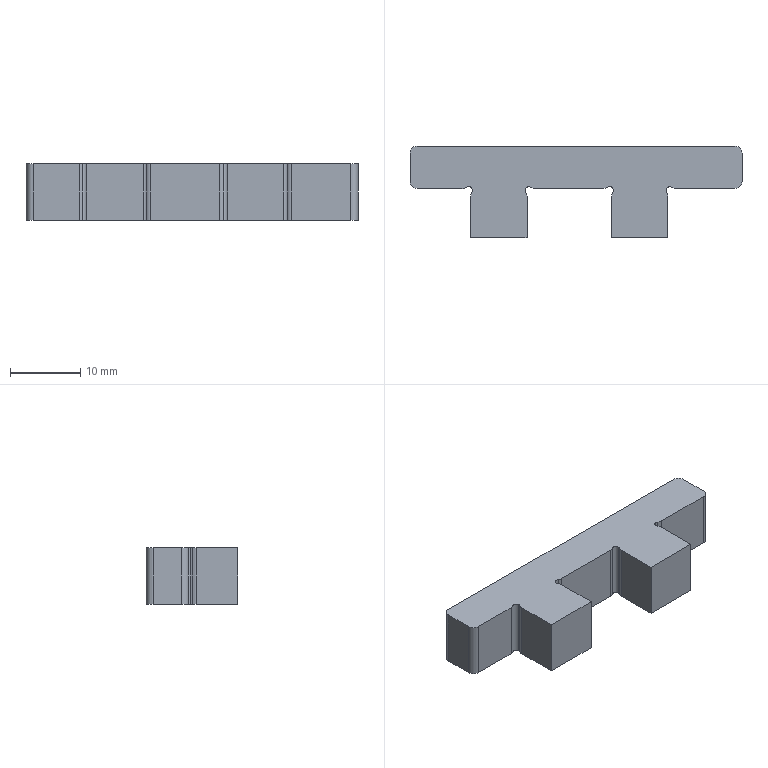Part | SolidWorks | features Fillet 1, FlatPattern 1, ICE 1, SMBaseFlange 1, SheetMetal 1 | 1 solid | 32 faces | box 47.1 x 13 x 8 mm | volume 3140 mm3 | cylinder 18 | plane 14 | commonest cylinder face diameters 2 x12 1 x6
STEP:
#1=CARTESIAN_POINT('',(-10.518,-33.899,0.));
#2=VERTEX_POINT('',#1);
#3=CARTESIAN_POINT('',(-11.295,-33.482,0.));
#4=VERTEX_POINT('',#3);
#5=CARTESIAN_POINT('',(-11.018,-33.899,0.));
#6=DIRECTION('',(0.,0.,1.));
#7=DIRECTION('',(1.,0.,0.));
#8=AXIS2_PLACEMENT_3D('',#5,#6,#7);
#9=CIRCLE('',#8,0.5);
#10=EDGE_CURVE('',#2,#4,#9,.T.);
#11=ORIENTED_EDGE('',*,*,#10,.F.);
#12=CARTESIAN_POINT('',(-10.518,-33.899,8.));
#13=VERTEX_POINT('',#12);
#14=CARTESIAN_POINT('',(-10.518,-33.899,0.));
#15=DIRECTION('',(0.,0.,1.));
#16=VECTOR('',#15,1000.);
#17=LINE('',#14,#16);
#18=EDGE_CURVE('',#2,#13,#17,.T.);
#19=ORIENTED_EDGE('',*,*,#18,.T.);
#20=CARTESIAN_POINT('',(-11.295,-33.482,8.));
#21=VERTEX_POINT('',#20);
#22=CARTESIAN_POINT('',(-11.018,-33.899,8.));
#23=DIRECTION('',(0.,0.,1.));
#24=DIRECTION('',(1.,0.,0.));
#25=AXIS2_PLACEMENT_3D('',#22,#23,#24);
#26=CIRCLE('',#25,0.5);
#27=EDGE_CURVE('',#13,#21,#26,.T.);
#28=ORIENTED_EDGE('',*,*,#27,.T.);
#29=CARTESIAN_POINT('',(-11.295,-33.482,0.));
#30=DIRECTION('',(0.,0.,-1.));
#31=VECTOR('',#30,1000.);
#32=LINE('',#29,#31);
#33=EDGE_CURVE('',#21,#4,#32,.T.);
#34=ORIENTED_EDGE('',*,*,#33,.T.);
#35=EDGE_LOOP('',(#11,#19,#28,#34));
#36=FACE_OUTER_BOUND('',#35,.T.);
#37=CARTESIAN_POINT('',(-11.018,-33.899,0.));
#38=DIRECTION('',(0.,0.,1.));
#39=DIRECTION('',(1.,0.,0.));
#40=AXIS2_PLACEMENT_3D('',#37,#38,#39);
#41=CYLINDRICAL_SURFACE('',#40,0.5);
#42=ADVANCED_FACE('',(#36),#41,.F.);
#43=CARTESIAN_POINT('',(9.482,-33.899,0.));
#44=VERTEX_POINT('',#43);
#45=CARTESIAN_POINT('',(8.705,-33.482,0.));
#46=VERTEX_POINT('',#45);
#47=CARTESIAN_POINT('',(8.982,-33.899,0.));
#48=DIRECTION('',(0.,0.,1.));
#49=DIRECTION('',(1.,0.,0.));
#50=AXIS2_PLACEMENT_3D('',#47,#48,#49);
#51=CIRCLE('',#50,0.5);
#52=EDGE_CURVE('',#44,#46,#51,.T.);
#53=ORIENTED_EDGE('',*,*,#52,.F.);
#54=CARTESIAN_POINT('',(9.482,-33.899,8.));
#55=VERTEX_POINT('',#54);
#56=CARTESIAN_POINT('',(9.482,-33.899,0.));
#57=DIRECTION('',(0.,0.,1.));
#58=VECTOR('',#57,1000.);
#59=LINE('',#56,#58);
#60=EDGE_CURVE('',#44,#55,#59,.T.);
#61=ORIENTED_EDGE('',*,*,#60,.T.);
#62=CARTESIAN_POINT('',(8.705,-33.482,8.));
#63=VERTEX_POINT('',#62);
#64=CARTESIAN_POINT('',(8.982,-33.899,8.));
#65=DIRECTION('',(0.,0.,1.));
#66=DIRECTION('',(1.,0.,0.));
#67=AXIS2_PLACEMENT_3D('',#64,#65,#66);
#68=CIRCLE('',#67,0.5);
#69=EDGE_CURVE('',#55,#63,#68,.T.);
#70=ORIENTED_EDGE('',*,*,#69,.T.);
#71=CARTESIAN_POINT('',(8.705,-33.482,0.));
#72=DIRECTION('',(0.,0.,-1.));
#73=VECTOR('',#72,1000.);
#74=LINE('',#71,#73);
#75=EDGE_CURVE('',#63,#46,#74,.T.);
#76=ORIENTED_EDGE('',*,*,#75,.T.);
#77=EDGE_LOOP('',(#53,#61,#70,#76));
#78=FACE_OUTER_BOUND('',#77,.T.);
#79=CARTESIAN_POINT('',(8.982,-33.899,0.));
#80=DIRECTION('',(0.,0.,1.));
#81=DIRECTION('',(1.,0.,0.));
#82=AXIS2_PLACEMENT_3D('',#79,#80,#81);
#83=CYLINDRICAL_SURFACE('',#82,0.5);
#84=ADVANCED_FACE('',(#78),#83,.F.);
#85=CARTESIAN_POINT('',(-18.368,-33.649,8.));
#86=VERTEX_POINT('',#85);
#87=CARTESIAN_POINT('',(-11.847,-33.649,8.));
#88=VERTEX_POINT('',#87);
#89=CARTESIAN_POINT('',(-10.768,-33.649,8.));
#90=DIRECTION('',(1.,0.,0.));
#91=VECTOR('',#90,1000.);
#92=LINE('',#89,#91);
#93=EDGE_CURVE('',#86,#88,#92,.T.);
#94=ORIENTED_EDGE('',*,*,#93,.F.);
#95=CARTESIAN_POINT('',(-18.368,-33.649,0.));
#96=VERTEX_POINT('',#95);
#97=CARTESIAN_POINT('',(-18.368,-33.649,8.));
#98=DIRECTION('',(0.,0.,-1.));
#99=VECTOR('',#98,1000.);
#100=LINE('',#97,#99);
#101=EDGE_CURVE('',#86,#96,#100,.T.);
#102=ORIENTED_EDGE('',*,*,#101,.T.);
#103=CARTESIAN_POINT('',(-11.847,-33.649,0.));
#104=VERTEX_POINT('',#103);
#105=CARTESIAN_POINT('',(-10.768,-33.649,0.));
#106=DIRECTION('',(1.,0.,0.));
#107=VECTOR('',#106,1000.);
#108=LINE('',#105,#107);
#109=EDGE_CURVE('',#96,#104,#108,.T.);
#110=ORIENTED_EDGE('',*,*,#109,.T.);
#111=CARTESIAN_POINT('',(-11.847,-33.649,8.));
#112=DIRECTION('',(0.,0.,1.));
#113=VECTOR('',#112,1000.);
#114=LINE('',#111,#113);
#115=EDGE_CURVE('',#104,#88,#114,.T.);
#116=ORIENTED_EDGE('',*,*,#115,.T.);
#117=EDGE_LOOP('',(#94,#102,#110,#116));
#118=FACE_OUTER_BOUND('',#117,.T.);
#119=CARTESIAN_POINT('',(-10.768,-33.649,8.));
#120=DIRECTION('',(0.,1.,0.));
#121=DIRECTION('',(0.,0.,1.));
#122=AXIS2_PLACEMENT_3D('',#119,#120,#121);
#123=PLANE('',#122);
#124=ADVANCED_FACE('',(#118),#123,.F.);
#125=CARTESIAN_POINT('',(-10.768,-34.728,8.));
#126=VERTEX_POINT('',#125);
#127=CARTESIAN_POINT('',(-10.768,-40.649,8.));
#128=VERTEX_POINT('',#127);
#129=CARTESIAN_POINT('',(-10.768,-40.649,8.));
#130=DIRECTION('',(0.,-1.,0.));
#131=VECTOR('',#130,1000.);
#132=LINE('',#129,#131);
#133=EDGE_CURVE('',#126,#128,#132,.T.);
#134=ORIENTED_EDGE('',*,*,#133,.F.);
#135=CARTESIAN_POINT('',(-10.768,-34.728,0.));
#136=VERTEX_POINT('',#135);
#137=CARTESIAN_POINT('',(-10.768,-34.728,0.));
#138=DIRECTION('',(0.,0.,-1.));
#139=VECTOR('',#138,1000.);
#140=LINE('',#137,#139);
#141=EDGE_CURVE('',#126,#136,#140,.T.);
#142=ORIENTED_EDGE('',*,*,#141,.T.);
#143=CARTESIAN_POINT('',(-10.768,-40.649,0.));
#144=VERTEX_POINT('',#143);
#145=CARTESIAN_POINT('',(-10.768,-40.649,0.));
#146=DIRECTION('',(0.,-1.,0.));
#147=VECTOR('',#146,1000.);
#148=LINE('',#145,#147);
#149=EDGE_CURVE('',#136,#144,#148,.T.);
#150=ORIENTED_EDGE('',*,*,#149,.T.);
#151=CARTESIAN_POINT('',(-10.768,-40.649,8.));
#152=DIRECTION('',(0.,0.,-1.));
#153=VECTOR('',#152,1000.);
#154=LINE('',#151,#153);
#155=EDGE_CURVE('',#128,#144,#154,.T.);
#156=ORIENTED_EDGE('',*,*,#155,.F.);
#157=EDGE_LOOP('',(#134,#142,#150,#156));
#158=FACE_OUTER_BOUND('',#157,.T.);
#159=CARTESIAN_POINT('',(-10.768,-40.649,8.));
#160=DIRECTION('',(1.,0.,0.));
#161=DIRECTION('',(0.,0.,-1.));
#162=AXIS2_PLACEMENT_3D('',#159,#160,#161);
#163=PLANE('',#162);
#164=ADVANCED_FACE('',(#158),#163,.F.);
#165=CARTESIAN_POINT('',(-2.768,-40.649,0.));
#166=VERTEX_POINT('',#165);
#167=CARTESIAN_POINT('',(-2.768,-34.728,0.));
#168=VERTEX_POINT('',#167);
#169=CARTESIAN_POINT('',(-2.768,-33.649,0.));
#170=DIRECTION('',(0.,1.,0.));
#171=VECTOR('',#170,1000.);
#172=LINE('',#169,#171);
#173=EDGE_CURVE('',#166,#168,#172,.T.);
#174=ORIENTED_EDGE('',*,*,#173,.T.);
#175=CARTESIAN_POINT('',(-2.768,-34.728,8.));
#176=VERTEX_POINT('',#175);
#177=CARTESIAN_POINT('',(-2.768,-34.728,8.));
#178=DIRECTION('',(0.,0.,1.));
#179=VECTOR('',#178,1000.);
#180=LINE('',#177,#179);
#181=EDGE_CURVE('',#168,#176,#180,.T.);
#182=ORIENTED_EDGE('',*,*,#181,.T.);
#183=CARTESIAN_POINT('',(-2.768,-40.649,8.));
#184=VERTEX_POINT('',#183);
#185=CARTESIAN_POINT('',(-2.768,-33.649,8.));
#186=DIRECTION('',(0.,1.,0.));
#187=VECTOR('',#186,1000.);
#188=LINE('',#185,#187);
#189=EDGE_CURVE('',#184,#176,#188,.T.);
#190=ORIENTED_EDGE('',*,*,#189,.F.);
#191=CARTESIAN_POINT('',(-2.768,-40.649,8.));
#192=DIRECTION('',(0.,0.,-1.));
#193=VECTOR('',#192,1000.);
#194=LINE('',#191,#193);
#195=EDGE_CURVE('',#184,#166,#194,.T.);
#196=ORIENTED_EDGE('',*,*,#195,.T.);
#197=EDGE_LOOP('',(#174,#182,#190,#196));
#198=FACE_OUTER_BOUND('',#197,.T.);
#199=CARTESIAN_POINT('',(-2.768,-33.649,8.));
#200=DIRECTION('',(-1.,0.,0.));
#201=DIRECTION('',(0.,0.,1.));
#202=AXIS2_PLACEMENT_3D('',#199,#200,#201);
#203=PLANE('',#202);
#204=ADVANCED_FACE('',(#198),#203,.F.);
#205=CARTESIAN_POINT('',(-1.689,-33.649,0.));
#206=VERTEX_POINT('',#205);
#207=CARTESIAN_POINT('',(8.153,-33.649,0.));
#208=VERTEX_POINT('',#207);
#209=CARTESIAN_POINT('',(9.232,-33.649,0.));
#210=DIRECTION('',(1.,0.,0.));
#211=VECTOR('',#210,1000.);
#212=LINE('',#209,#211);
#213=EDGE_CURVE('',#206,#208,#212,.T.);
#214=ORIENTED_EDGE('',*,*,#213,.T.);
#215=CARTESIAN_POINT('',(8.153,-33.649,8.));
#216=VERTEX_POINT('',#215);
#217=CARTESIAN_POINT('',(8.153,-33.649,8.));
#218=DIRECTION('',(0.,0.,1.));
#219=VECTOR('',#218,1000.);
#220=LINE('',#217,#219);
#221=EDGE_CURVE('',#208,#216,#220,.T.);
#222=ORIENTED_EDGE('',*,*,#221,.T.);
#223=CARTESIAN_POINT('',(-1.689,-33.649,8.));
#224=VERTEX_POINT('',#223);
#225=CARTESIAN_POINT('',(9.232,-33.649,8.));
#226=DIRECTION('',(1.,0.,0.));
#227=VECTOR('',#226,1000.);
#228=LINE('',#225,#227);
#229=EDGE_CURVE('',#224,#216,#228,.T.);
#230=ORIENTED_EDGE('',*,*,#229,.F.);
#231=CARTESIAN_POINT('',(-1.689,-33.649,0.));
#232=DIRECTION('',(0.,0.,-1.));
#233=VECTOR('',#232,1000.);
#234=LINE('',#231,#233);
#235=EDGE_CURVE('',#224,#206,#234,.T.);
#236=ORIENTED_EDGE('',*,*,#235,.T.);
#237=EDGE_LOOP('',(#214,#222,#230,#236));
#238=FACE_OUTER_BOUND('',#237,.T.);
#239=CARTESIAN_POINT('',(9.232,-33.649,8.));
#240=DIRECTION('',(0.,1.,0.));
#241=DIRECTION('',(0.,0.,1.));
#242=AXIS2_PLACEMENT_3D('',#239,#240,#241);
#243=PLANE('',#242);
#244=ADVANCED_FACE('',(#238),#243,.F.);
#245=CARTESIAN_POINT('',(9.232,-34.728,8.));
#246=VERTEX_POINT('',#245);
#247=CARTESIAN_POINT('',(9.232,-40.649,8.));
#248=VERTEX_POINT('',#247);
#249=CARTESIAN_POINT('',(9.232,-40.649,8.));
#250=DIRECTION('',(0.,-1.,0.));
#251=VECTOR('',#250,1000.);
#252=LINE('',#249,#251);
#253=EDGE_CURVE('',#246,#248,#252,.T.);
#254=ORIENTED_EDGE('',*,*,#253,.F.);
#255=CARTESIAN_POINT('',(9.232,-34.728,0.));
#256=VERTEX_POINT('',#255);
#257=CARTESIAN_POINT('',(9.232,-34.728,0.));
#258=DIRECTION('',(0.,0.,-1.));
#259=VECTOR('',#258,1000.);
#260=LINE('',#257,#259);
#261=EDGE_CURVE('',#246,#256,#260,.T.);
#262=ORIENTED_EDGE('',*,*,#261,.T.);
#263=CARTESIAN_POINT('',(9.232,-40.649,0.));
#264=VERTEX_POINT('',#263);
#265=CARTESIAN_POINT('',(9.232,-40.649,0.));
#266=DIRECTION('',(0.,-1.,0.));
#267=VECTOR('',#266,1000.);
#268=LINE('',#265,#267);
#269=EDGE_CURVE('',#256,#264,#268,.T.);
#270=ORIENTED_EDGE('',*,*,#269,.T.);
#271=CARTESIAN_POINT('',(9.232,-40.649,8.));
#272=DIRECTION('',(0.,0.,-1.));
#273=VECTOR('',#272,1000.);
#274=LINE('',#271,#273);
#275=EDGE_CURVE('',#248,#264,#274,.T.);
#276=ORIENTED_EDGE('',*,*,#275,.F.);
#277=EDGE_LOOP('',(#254,#262,#270,#276));
#278=FACE_OUTER_BOUND('',#277,.T.);
#279=CARTESIAN_POINT('',(9.232,-40.649,8.));
#280=DIRECTION('',(1.,0.,0.));
#281=DIRECTION('',(0.,0.,-1.));
#282=AXIS2_PLACEMENT_3D('',#279,#280,#281);
#283=PLANE('',#282);
#284=ADVANCED_FACE('',(#278),#283,.F.);
#285=CARTESIAN_POINT('',(17.232,-40.649,0.));
#286=VERTEX_POINT('',#285);
#287=CARTESIAN_POINT('',(17.232,-34.728,0.));
#288=VERTEX_POINT('',#287);
#289=CARTESIAN_POINT('',(17.232,-33.649,0.));
#290=DIRECTION('',(0.,1.,0.));
#291=VECTOR('',#290,1000.);
#292=LINE('',#289,#291);
#293=EDGE_CURVE('',#286,#288,#292,.T.);
#294=ORIENTED_EDGE('',*,*,#293,.T.);
#295=CARTESIAN_POINT('',(17.232,-34.728,8.));
#296=VERTEX_POINT('',#295);
#297=CARTESIAN_POINT('',(17.232,-34.728,8.));
#298=DIRECTION('',(0.,0.,1.));
#299=VECTOR('',#298,1000.);
#300=LINE('',#297,#299);
#301=EDGE_CURVE('',#288,#296,#300,.T.);
#302=ORIENTED_EDGE('',*,*,#301,.T.);
#303=CARTESIAN_POINT('',(17.232,-40.649,8.));
#304=VERTEX_POINT('',#303);
#305=CARTESIAN_POINT('',(17.232,-33.649,8.));
#306=DIRECTION('',(0.,1.,0.));
#307=VECTOR('',#306,1000.);
#308=LINE('',#305,#307);
#309=EDGE_CURVE('',#304,#296,#308,.T.);
#310=ORIENTED_EDGE('',*,*,#309,.F.);
#311=CARTESIAN_POINT('',(17.232,-40.649,8.));
#312=DIRECTION('',(0.,0.,-1.));
#313=VECTOR('',#312,1000.);
#314=LINE('',#311,#313);
#315=EDGE_CURVE('',#304,#286,#314,.T.);
#316=ORIENTED_EDGE('',*,*,#315,.T.);
#317=EDGE_LOOP('',(#294,#302,#310,#316));
#318=FACE_OUTER_BOUND('',#317,.T.);
#319=CARTESIAN_POINT('',(17.232,-33.649,8.));
#320=DIRECTION('',(-1.,0.,0.));
#321=DIRECTION('',(0.,0.,1.));
#322=AXIS2_PLACEMENT_3D('',#319,#320,#321);
#323=PLANE('',#322);
#324=ADVANCED_FACE('',(#318),#323,.F.);
#325=CARTESIAN_POINT('',(18.311,-33.649,0.));
#326=VERTEX_POINT('',#325);
#327=CARTESIAN_POINT('',(26.732,-33.649,0.));
#328=VERTEX_POINT('',#327);
#329=CARTESIAN_POINT('',(27.732,-33.649,0.));
#330=DIRECTION('',(1.,0.,0.));
#331=VECTOR('',#330,1000.);
#332=LINE('',#329,#331);
#333=EDGE_CURVE('',#326,#328,#332,.T.);
#334=ORIENTED_EDGE('',*,*,#333,.T.);
#335=CARTESIAN_POINT('',(26.732,-33.649,8.));
#336=VERTEX_POINT('',#335);
#337=CARTESIAN_POINT('',(26.732,-33.649,8.));
#338=DIRECTION('',(0.,0.,1.));
#339=VECTOR('',#338,1000.);
#340=LINE('',#337,#339);
#341=EDGE_CURVE('',#328,#336,#340,.T.);
#342=ORIENTED_EDGE('',*,*,#341,.T.);
#343=CARTESIAN_POINT('',(18.311,-33.649,8.));
#344=VERTEX_POINT('',#343);
#345=CARTESIAN_POINT('',(27.732,-33.649,8.));
#346=DIRECTION('',(1.,0.,0.));
#347=VECTOR('',#346,1000.);
#348=LINE('',#345,#347);
#349=EDGE_CURVE('',#344,#336,#348,.T.);
#350=ORIENTED_EDGE('',*,*,#349,.F.);
#351=CARTESIAN_POINT('',(18.311,-33.649,0.));
#352=DIRECTION('',(0.,0.,-1.));
#353=VECTOR('',#352,1000.);
#354=LINE('',#351,#353);
#355=EDGE_CURVE('',#344,#326,#354,.T.);
#356=ORIENTED_EDGE('',*,*,#355,.T.);
#357=EDGE_LOOP('',(#334,#342,#350,#356));
#358=FACE_OUTER_BOUND('',#357,.T.);
#359=CARTESIAN_POINT('',(27.732,-33.649,8.));
#360=DIRECTION('',(0.,1.,0.));
#361=DIRECTION('',(0.,0.,1.));
#362=AXIS2_PLACEMENT_3D('',#359,#360,#361);
#363=PLANE('',#362);
#364=ADVANCED_FACE('',(#358),#363,.F.);
#365=ORIENTED_EDGE('',*,*,#349,.T.);
#366=CARTESIAN_POINT('',(27.732,-32.649,8.));
#367=VERTEX_POINT('',#366);
#368=CARTESIAN_POINT('',(26.732,-32.649,8.));
#369=DIRECTION('',(0.,0.,1.));
#370=DIRECTION('',(1.,0.,0.));
#371=AXIS2_PLACEMENT_3D('',#368,#369,#370);
#372=CIRCLE('',#371,1.);
#373=EDGE_CURVE('',#336,#367,#372,.T.);
#374=ORIENTED_EDGE('',*,*,#373,.T.);
#375=CARTESIAN_POINT('',(27.732,-28.649,8.));
#376=VERTEX_POINT('',#375);
#377=CARTESIAN_POINT('',(27.732,-27.649,8.));
#378=DIRECTION('',(0.,1.,0.));
#379=VECTOR('',#378,1000.);
#380=LINE('',#377,#379);
#381=EDGE_CURVE('',#367,#376,#380,.T.);
#382=ORIENTED_EDGE('',*,*,#381,.T.);
#383=CARTESIAN_POINT('',(26.732,-27.649,8.));
#384=VERTEX_POINT('',#383);
#385=CARTESIAN_POINT('',(26.732,-28.649,8.));
#386=DIRECTION('',(0.,0.,1.));
#387=DIRECTION('',(1.,0.,0.));
#388=AXIS2_PLACEMENT_3D('',#385,#386,#387);
#389=CIRCLE('',#388,1.);
#390=EDGE_CURVE('',#376,#384,#389,.T.);
#391=ORIENTED_EDGE('',*,*,#390,.T.);
#392=CARTESIAN_POINT('',(-18.368,-27.649,8.));
#393=VERTEX_POINT('',#392);
#394=CARTESIAN_POINT('',(-19.368,-27.649,8.));
#395=DIRECTION('',(-1.,0.,0.));
#396=VECTOR('',#395,1000.);
#397=LINE('',#394,#396);
#398=EDGE_CURVE('',#384,#393,#397,.T.);
#399=ORIENTED_EDGE('',*,*,#398,.T.);
#400=CARTESIAN_POINT('',(-19.368,-28.649,8.));
#401=VERTEX_POINT('',#400);
#402=CARTESIAN_POINT('',(-18.368,-28.649,8.));
#403=DIRECTION('',(0.,0.,1.));
#404=DIRECTION('',(1.,0.,0.));
#405=AXIS2_PLACEMENT_3D('',#402,#403,#404);
#406=CIRCLE('',#405,1.);
#407=EDGE_CURVE('',#393,#401,#406,.T.);
#408=ORIENTED_EDGE('',*,*,#407,.T.);
#409=CARTESIAN_POINT('',(-19.368,-32.649,8.));
#410=VERTEX_POINT('',#409);
#411=CARTESIAN_POINT('',(-19.368,-33.649,8.));
#412=DIRECTION('',(0.000001026,-1.,0.));
#413=VECTOR('',#412,1000.);
#414=LINE('',#411,#413);
#415=EDGE_CURVE('',#401,#410,#414,.T.);
#416=ORIENTED_EDGE('',*,*,#415,.T.);
#417=CARTESIAN_POINT('',(-18.368,-32.649,8.));
#418=DIRECTION('',(0.,0.,1.));
#419=DIRECTION('',(1.,0.,0.));
#420=AXIS2_PLACEMENT_3D('',#417,#418,#419);
#421=CIRCLE('',#420,1.);
#422=EDGE_CURVE('',#410,#86,#421,.T.);
#423=ORIENTED_EDGE('',*,*,#422,.T.);
#424=ORIENTED_EDGE('',*,*,#93,.T.);
#425=CARTESIAN_POINT('',(-11.847,-32.649,8.));
#426=DIRECTION('',(0.,0.,1.));
#427=DIRECTION('',(1.,0.,0.));
#428=AXIS2_PLACEMENT_3D('',#425,#426,#427);
#429=CIRCLE('',#428,1.);
#430=EDGE_CURVE('',#88,#21,#429,.T.);
#431=ORIENTED_EDGE('',*,*,#430,.T.);
#432=ORIENTED_EDGE('',*,*,#27,.F.);
#433=CARTESIAN_POINT('',(-10.602,-34.175,8.));
#434=VERTEX_POINT('',#433);
#435=CARTESIAN_POINT('',(-11.018,-33.899,8.));
#436=DIRECTION('',(0.,0.,1.));
#437=DIRECTION('',(1.,0.,0.));
#438=AXIS2_PLACEMENT_3D('',#435,#436,#437);
#439=CIRCLE('',#438,0.5);
#440=EDGE_CURVE('',#434,#13,#439,.T.);
#441=ORIENTED_EDGE('',*,*,#440,.F.);
#442=CARTESIAN_POINT('',(-9.768,-34.728,8.));
#443=DIRECTION('',(0.,0.,1.));
#444=DIRECTION('',(1.,0.,0.));
#445=AXIS2_PLACEMENT_3D('',#442,#443,#444);
#446=CIRCLE('',#445,1.);
#447=EDGE_CURVE('',#434,#126,#446,.T.);
#448=ORIENTED_EDGE('',*,*,#447,.T.);
#449=ORIENTED_EDGE('',*,*,#133,.T.);
#450=CARTESIAN_POINT('',(-2.768,-40.649,8.));
#451=DIRECTION('',(1.,0.,0.));
#452=VECTOR('',#451,1000.);
#453=LINE('',#450,#452);
#454=EDGE_CURVE('',#128,#184,#453,.T.);
#455=ORIENTED_EDGE('',*,*,#454,.T.);
#456=ORIENTED_EDGE('',*,*,#189,.T.);
#457=CARTESIAN_POINT('',(-2.935,-34.175,8.));
#458=VERTEX_POINT('',#457);
#459=CARTESIAN_POINT('',(-3.768,-34.728,8.));
#460=DIRECTION('',(0.,0.,1.));
#461=DIRECTION('',(1.,0.,0.));
#462=AXIS2_PLACEMENT_3D('',#459,#460,#461);
#463=CIRCLE('',#462,1.);
#464=EDGE_CURVE('',#176,#458,#463,.T.);
#465=ORIENTED_EDGE('',*,*,#464,.T.);
#466=CARTESIAN_POINT('',(-2.242,-33.482,8.));
#467=VERTEX_POINT('',#466);
#468=CARTESIAN_POINT('',(-2.518,-33.899,8.));
#469=DIRECTION('',(0.,0.,1.));
#470=DIRECTION('',(1.,0.,0.));
#471=AXIS2_PLACEMENT_3D('',#468,#469,#470);
#472=CIRCLE('',#471,0.5);
#473=EDGE_CURVE('',#467,#458,#472,.T.);
#474=ORIENTED_EDGE('',*,*,#473,.F.);
#475=CARTESIAN_POINT('',(-1.689,-32.649,8.));
#476=DIRECTION('',(0.,0.,1.));
#477=DIRECTION('',(1.,0.,0.));
#478=AXIS2_PLACEMENT_3D('',#475,#476,#477);
#479=CIRCLE('',#478,1.);
#480=EDGE_CURVE('',#467,#224,#479,.T.);
#481=ORIENTED_EDGE('',*,*,#480,.T.);
#482=ORIENTED_EDGE('',*,*,#229,.T.);
#483=CARTESIAN_POINT('',(8.153,-32.649,8.));
#484=DIRECTION('',(0.,0.,1.));
#485=DIRECTION('',(1.,0.,0.));
#486=AXIS2_PLACEMENT_3D('',#483,#484,#485);
#487=CIRCLE('',#486,1.);
#488=EDGE_CURVE('',#216,#63,#487,.T.);
#489=ORIENTED_EDGE('',*,*,#488,.T.);
#490=ORIENTED_EDGE('',*,*,#69,.F.);
#491=CARTESIAN_POINT('',(9.398,-34.175,8.));
#492=VERTEX_POINT('',#491);
#493=CARTESIAN_POINT('',(8.982,-33.899,8.));
#494=DIRECTION('',(0.,0.,1.));
#495=DIRECTION('',(1.,0.,0.));
#496=AXIS2_PLACEMENT_3D('',#493,#494,#495);
#497=CIRCLE('',#496,0.5);
#498=EDGE_CURVE('',#492,#55,#497,.T.);
#499=ORIENTED_EDGE('',*,*,#498,.F.);
#500=CARTESIAN_POINT('',(10.232,-34.728,8.));
#501=DIRECTION('',(0.,0.,1.));
#502=DIRECTION('',(1.,0.,0.));
#503=AXIS2_PLACEMENT_3D('',#500,#501,#502);
#504=CIRCLE('',#503,1.);
#505=EDGE_CURVE('',#492,#246,#504,.T.);
#506=ORIENTED_EDGE('',*,*,#505,.T.);
#507=ORIENTED_EDGE('',*,*,#253,.T.);
#508=CARTESIAN_POINT('',(17.232,-40.649,8.));
#509=DIRECTION('',(1.,0.,0.));
#510=VECTOR('',#509,1000.);
#511=LINE('',#508,#510);
#512=EDGE_CURVE('',#248,#304,#511,.T.);
#513=ORIENTED_EDGE('',*,*,#512,.T.);
#514=ORIENTED_EDGE('',*,*,#309,.T.);
#515=CARTESIAN_POINT('',(17.065,-34.175,8.));
#516=VERTEX_POINT('',#515);
#517=CARTESIAN_POINT('',(16.232,-34.728,8.));
#518=DIRECTION('',(0.,0.,1.));
#519=DIRECTION('',(1.,0.,0.));
#520=AXIS2_PLACEMENT_3D('',#517,#518,#519);
#521=CIRCLE('',#520,1.);
#522=EDGE_CURVE('',#296,#516,#521,.T.);
#523=ORIENTED_EDGE('',*,*,#522,.T.);
#524=CARTESIAN_POINT('',(17.758,-33.482,8.));
#525=VERTEX_POINT('',#524);
#526=CARTESIAN_POINT('',(17.482,-33.899,8.));
#527=DIRECTION('',(0.,0.,1.));
#528=DIRECTION('',(1.,0.,0.));
#529=AXIS2_PLACEMENT_3D('',#526,#527,#528);
#530=CIRCLE('',#529,0.5);
#531=EDGE_CURVE('',#525,#516,#530,.T.);
#532=ORIENTED_EDGE('',*,*,#531,.F.);
#533=CARTESIAN_POINT('',(18.311,-32.649,8.));
#534=DIRECTION('',(0.,0.,1.));
#535=DIRECTION('',(1.,0.,0.));
#536=AXIS2_PLACEMENT_3D('',#533,#534,#535);
#537=CIRCLE('',#536,1.);
#538=EDGE_CURVE('',#525,#344,#537,.T.);
#539=ORIENTED_EDGE('',*,*,#538,.T.);
#540=EDGE_LOOP('',(#365,#374,#382,#391,#399,#408,#416,#423,#424,#431,#432,#441,#448,#449,#455,#456,#465,#474,#481,#482,#489,#490,#499,#506,#507,#513,#514,#523,#532,#539));
#541=FACE_OUTER_BOUND('',#540,.T.);
#542=CARTESIAN_POINT('',(0.,0.,8.));
#543=DIRECTION('',(0.,0.,1.));
#544=DIRECTION('',(1.,0.,0.));
#545=AXIS2_PLACEMENT_3D('',#542,#543,#544);
#546=PLANE('',#545);
#547=ADVANCED_FACE('',(#541),#546,.T.);
#548=CARTESIAN_POINT('',(27.732,-32.649,0.));
#549=VERTEX_POINT('',#548);
#550=CARTESIAN_POINT('',(27.732,-28.649,0.));
#551=VERTEX_POINT('',#550);
#552=CARTESIAN_POINT('',(27.732,-27.649,0.));
#553=DIRECTION('',(0.,1.,0.));
#554=VECTOR('',#553,1000.);
#555=LINE('',#552,#554);
#556=EDGE_CURVE('',#549,#551,#555,.T.);
#557=ORIENTED_EDGE('',*,*,#556,.F.);
#558=CARTESIAN_POINT('',(26.732,-32.649,0.));
#559=DIRECTION('',(0.,0.,-1.));
#560=DIRECTION('',(1.,0.,0.));
#561=AXIS2_PLACEMENT_3D('',#558,#559,#560);
#562=CIRCLE('',#561,1.);
#563=EDGE_CURVE('',#549,#328,#562,.T.);
#564=ORIENTED_EDGE('',*,*,#563,.T.);
#565=ORIENTED_EDGE('',*,*,#333,.F.);
#566=CARTESIAN_POINT('',(17.758,-33.482,0.));
#567=VERTEX_POINT('',#566);
#568=CARTESIAN_POINT('',(18.311,-32.649,0.));
#569=DIRECTION('',(0.,0.,-1.));
#570=DIRECTION('',(1.,0.,0.));
#571=AXIS2_PLACEMENT_3D('',#568,#569,#570);
#572=CIRCLE('',#571,1.);
#573=EDGE_CURVE('',#326,#567,#572,.T.);
#574=ORIENTED_EDGE('',*,*,#573,.T.);
#575=CARTESIAN_POINT('',(17.065,-34.175,0.));
#576=VERTEX_POINT('',#575);
#577=CARTESIAN_POINT('',(17.482,-33.899,0.));
#578=DIRECTION('',(0.,0.,1.));
#579=DIRECTION('',(1.,0.,0.));
#580=AXIS2_PLACEMENT_3D('',#577,#578,#579);
#581=CIRCLE('',#580,0.5);
#582=EDGE_CURVE('',#567,#576,#581,.T.);
#583=ORIENTED_EDGE('',*,*,#582,.T.);
#584=CARTESIAN_POINT('',(16.232,-34.728,0.));
#585=DIRECTION('',(0.,0.,-1.));
#586=DIRECTION('',(1.,0.,0.));
#587=AXIS2_PLACEMENT_3D('',#584,#585,#586);
#588=CIRCLE('',#587,1.);
#589=EDGE_CURVE('',#576,#288,#588,.T.);
#590=ORIENTED_EDGE('',*,*,#589,.T.);
#591=ORIENTED_EDGE('',*,*,#293,.F.);
#592=CARTESIAN_POINT('',(17.232,-40.649,0.));
#593=DIRECTION('',(1.,0.,0.));
#594=VECTOR('',#593,1000.);
#595=LINE('',#592,#594);
#596=EDGE_CURVE('',#264,#286,#595,.T.);
#597=ORIENTED_EDGE('',*,*,#596,.F.);
#598=ORIENTED_EDGE('',*,*,#269,.F.);
#599=CARTESIAN_POINT('',(9.398,-34.175,0.));
#600=VERTEX_POINT('',#599);
#601=CARTESIAN_POINT('',(10.232,-34.728,0.));
#602=DIRECTION('',(0.,0.,-1.));
#603=DIRECTION('',(1.,0.,0.));
#604=AXIS2_PLACEMENT_3D('',#601,#602,#603);
#605=CIRCLE('',#604,1.);
#606=EDGE_CURVE('',#256,#600,#605,.T.);
#607=ORIENTED_EDGE('',*,*,#606,.T.);
#608=CARTESIAN_POINT('',(8.982,-33.899,0.));
#609=DIRECTION('',(0.,0.,1.));
#610=DIRECTION('',(1.,0.,0.));
#611=AXIS2_PLACEMENT_3D('',#608,#609,#610);
#612=CIRCLE('',#611,0.5);
#613=EDGE_CURVE('',#600,#44,#612,.T.);
#614=ORIENTED_EDGE('',*,*,#613,.T.);
#615=ORIENTED_EDGE('',*,*,#52,.T.);
#616=CARTESIAN_POINT('',(8.153,-32.649,0.));
#617=DIRECTION('',(0.,0.,-1.));
#618=DIRECTION('',(1.,0.,0.));
#619=AXIS2_PLACEMENT_3D('',#616,#617,#618);
#620=CIRCLE('',#619,1.);
#621=EDGE_CURVE('',#46,#208,#620,.T.);
#622=ORIENTED_EDGE('',*,*,#621,.T.);
#623=ORIENTED_EDGE('',*,*,#213,.F.);
#624=CARTESIAN_POINT('',(-2.242,-33.482,0.));
#625=VERTEX_POINT('',#624);
#626=CARTESIAN_POINT('',(-1.689,-32.649,0.));
#627=DIRECTION('',(0.,0.,-1.));
#628=DIRECTION('',(1.,0.,0.));
#629=AXIS2_PLACEMENT_3D('',#626,#627,#628);
#630=CIRCLE('',#629,1.);
#631=EDGE_CURVE('',#206,#625,#630,.T.);
#632=ORIENTED_EDGE('',*,*,#631,.T.);
#633=CARTESIAN_POINT('',(-2.935,-34.175,0.));
#634=VERTEX_POINT('',#633);
#635=CARTESIAN_POINT('',(-2.518,-33.899,0.));
#636=DIRECTION('',(0.,0.,1.));
#637=DIRECTION('',(1.,0.,0.));
#638=AXIS2_PLACEMENT_3D('',#635,#636,#637);
#639=CIRCLE('',#638,0.5);
#640=EDGE_CURVE('',#625,#634,#639,.T.);
#641=ORIENTED_EDGE('',*,*,#640,.T.);
#642=CARTESIAN_POINT('',(-3.768,-34.728,0.));
#643=DIRECTION('',(0.,0.,-1.));
#644=DIRECTION('',(1.,0.,0.));
#645=AXIS2_PLACEMENT_3D('',#642,#643,#644);
#646=CIRCLE('',#645,1.);
#647=EDGE_CURVE('',#634,#168,#646,.T.);
#648=ORIENTED_EDGE('',*,*,#647,.T.);
#649=ORIENTED_EDGE('',*,*,#173,.F.);
#650=CARTESIAN_POINT('',(-2.768,-40.649,0.));
#651=DIRECTION('',(1.,0.,0.));
#652=VECTOR('',#651,1000.);
#653=LINE('',#650,#652);
#654=EDGE_CURVE('',#144,#166,#653,.T.);
#655=ORIENTED_EDGE('',*,*,#654,.F.);
#656=ORIENTED_EDGE('',*,*,#149,.F.);
#657=CARTESIAN_POINT('',(-10.602,-34.175,0.));
#658=VERTEX_POINT('',#657);
#659=CARTESIAN_POINT('',(-9.768,-34.728,0.));
#660=DIRECTION('',(0.,0.,-1.));
#661=DIRECTION('',(1.,0.,0.));
#662=AXIS2_PLACEMENT_3D('',#659,#660,#661);
#663=CIRCLE('',#662,1.);
#664=EDGE_CURVE('',#136,#658,#663,.T.);
#665=ORIENTED_EDGE('',*,*,#664,.T.);
#666=CARTESIAN_POINT('',(-11.018,-33.899,0.));
#667=DIRECTION('',(0.,0.,1.));
#668=DIRECTION('',(1.,0.,0.));
#669=AXIS2_PLACEMENT_3D('',#666,#667,#668);
#670=CIRCLE('',#669,0.5);
#671=EDGE_CURVE('',#658,#2,#670,.T.);
#672=ORIENTED_EDGE('',*,*,#671,.T.);
#673=ORIENTED_EDGE('',*,*,#10,.T.);
#674=CARTESIAN_POINT('',(-11.847,-32.649,0.));
#675=DIRECTION('',(0.,0.,-1.));
#676=DIRECTION('',(1.,0.,0.));
#677=AXIS2_PLACEMENT_3D('',#674,#675,#676);
#678=CIRCLE('',#677,1.);
#679=EDGE_CURVE('',#4,#104,#678,.T.);
#680=ORIENTED_EDGE('',*,*,#679,.T.);
#681=ORIENTED_EDGE('',*,*,#109,.F.);
#682=CARTESIAN_POINT('',(-19.368,-32.649,0.));
#683=VERTEX_POINT('',#682);
#684=CARTESIAN_POINT('',(-18.368,-32.649,0.));
#685=DIRECTION('',(0.,0.,-1.));
#686=DIRECTION('',(1.,0.,0.));
#687=AXIS2_PLACEMENT_3D('',#684,#685,#686);
#688=CIRCLE('',#687,1.);
#689=EDGE_CURVE('',#96,#683,#688,.T.);
#690=ORIENTED_EDGE('',*,*,#689,.T.);
#691=CARTESIAN_POINT('',(-19.368,-28.649,0.));
#692=VERTEX_POINT('',#691);
#693=CARTESIAN_POINT('',(-19.368,-33.649,0.));
#694=DIRECTION('',(0.000001026,-1.,0.));
#695=VECTOR('',#694,1000.);
#696=LINE('',#693,#695);
#697=EDGE_CURVE('',#692,#683,#696,.T.);
#698=ORIENTED_EDGE('',*,*,#697,.F.);
#699=CARTESIAN_POINT('',(-18.368,-27.649,0.));
#700=VERTEX_POINT('',#699);
#701=CARTESIAN_POINT('',(-18.368,-28.649,0.));
#702=DIRECTION('',(0.,0.,-1.));
#703=DIRECTION('',(1.,0.,0.));
#704=AXIS2_PLACEMENT_3D('',#701,#702,#703);
#705=CIRCLE('',#704,1.);
#706=EDGE_CURVE('',#692,#700,#705,.T.);
#707=ORIENTED_EDGE('',*,*,#706,.T.);
#708=CARTESIAN_POINT('',(26.732,-27.649,0.));
#709=VERTEX_POINT('',#708);
#710=CARTESIAN_POINT('',(-19.368,-27.649,0.));
#711=DIRECTION('',(-1.,0.,0.));
#712=VECTOR('',#711,1000.);
#713=LINE('',#710,#712);
#714=EDGE_CURVE('',#709,#700,#713,.T.);
#715=ORIENTED_EDGE('',*,*,#714,.F.);
#716=CARTESIAN_POINT('',(26.732,-28.649,0.));
#717=DIRECTION('',(0.,0.,-1.));
#718=DIRECTION('',(1.,0.,0.));
#719=AXIS2_PLACEMENT_3D('',#716,#717,#718);
#720=CIRCLE('',#719,1.);
#721=EDGE_CURVE('',#709,#551,#720,.T.);
#722=ORIENTED_EDGE('',*,*,#721,.T.);
#723=EDGE_LOOP('',(#557,#564,#565,#574,#583,#590,#591,#597,#598,#607,#614,#615,#622,#623,#632,#641,#648,#649,#655,#656,#665,#672,#673,#680,#681,#690,#698,#707,#715,#722));
#724=FACE_OUTER_BOUND('',#723,.T.);
#725=CARTESIAN_POINT('',(0.,0.,0.));
#726=DIRECTION('',(0.,0.,1.));
#727=DIRECTION('',(1.,0.,0.));
#728=AXIS2_PLACEMENT_3D('',#725,#726,#727);
#729=PLANE('',#728);
#730=ADVANCED_FACE('',(#724),#729,.F.);
#731=ORIENTED_EDGE('',*,*,#654,.T.);
#732=ORIENTED_EDGE('',*,*,#195,.F.);
#733=ORIENTED_EDGE('',*,*,#454,.F.);
#734=ORIENTED_EDGE('',*,*,#155,.T.);
#735=EDGE_LOOP('',(#731,#732,#733,#734));
#736=FACE_OUTER_BOUND('',#735,.T.);
#737=CARTESIAN_POINT('',(-2.768,-40.649,8.));
#738=DIRECTION('',(0.,1.,0.));
#739=DIRECTION('',(0.,0.,1.));
#740=AXIS2_PLACEMENT_3D('',#737,#738,#739);
#741=PLANE('',#740);
#742=ADVANCED_FACE('',(#736),#741,.F.);
#743=ORIENTED_EDGE('',*,*,#596,.T.);
#744=ORIENTED_EDGE('',*,*,#315,.F.);
#745=ORIENTED_EDGE('',*,*,#512,.F.);
#746=ORIENTED_EDGE('',*,*,#275,.T.);
#747=EDGE_LOOP('',(#743,#744,#745,#746));
#748=FACE_OUTER_BOUND('',#747,.T.);
#749=CARTESIAN_POINT('',(17.232,-40.649,8.));
#750=DIRECTION('',(0.,1.,0.));
#751=DIRECTION('',(0.,0.,1.));
#752=AXIS2_PLACEMENT_3D('',#749,#750,#751);
#753=PLANE('',#752);
#754=ADVANCED_FACE('',(#748),#753,.F.);
#755=ORIENTED_EDGE('',*,*,#381,.F.);
#756=CARTESIAN_POINT('',(27.732,-32.649,8.));
#757=DIRECTION('',(0.,0.,-1.));
#758=VECTOR('',#757,1000.);
#759=LINE('',#756,#758);
#760=EDGE_CURVE('',#367,#549,#759,.T.);
#761=ORIENTED_EDGE('',*,*,#760,.T.);
#762=ORIENTED_EDGE('',*,*,#556,.T.);
#763=CARTESIAN_POINT('',(27.732,-28.649,8.));
#764=DIRECTION('',(0.,0.,1.));
#765=VECTOR('',#764,1000.);
#766=LINE('',#763,#765);
#767=EDGE_CURVE('',#551,#376,#766,.T.);
#768=ORIENTED_EDGE('',*,*,#767,.T.);
#769=EDGE_LOOP('',(#755,#761,#762,#768));
#770=FACE_OUTER_BOUND('',#769,.T.);
#771=CARTESIAN_POINT('',(27.732,-27.649,8.));
#772=DIRECTION('',(-1.,0.,0.));
#773=DIRECTION('',(0.,0.,1.));
#774=AXIS2_PLACEMENT_3D('',#771,#772,#773);
#775=PLANE('',#774);
#776=ADVANCED_FACE('',(#770),#775,.F.);
#777=ORIENTED_EDGE('',*,*,#398,.F.);
#778=CARTESIAN_POINT('',(26.732,-27.649,8.));
#779=DIRECTION('',(0.,0.,-1.));
#780=VECTOR('',#779,1000.);
#781=LINE('',#778,#780);
#782=EDGE_CURVE('',#384,#709,#781,.T.);
#783=ORIENTED_EDGE('',*,*,#782,.T.);
#784=ORIENTED_EDGE('',*,*,#714,.T.);
#785=CARTESIAN_POINT('',(-18.368,-27.649,8.));
#786=DIRECTION('',(0.,0.,1.));
#787=VECTOR('',#786,1000.);
#788=LINE('',#785,#787);
#789=EDGE_CURVE('',#700,#393,#788,.T.);
#790=ORIENTED_EDGE('',*,*,#789,.T.);
#791=EDGE_LOOP('',(#777,#783,#784,#790));
#792=FACE_OUTER_BOUND('',#791,.T.);
#793=CARTESIAN_POINT('',(-19.368,-27.649,8.));
#794=DIRECTION('',(0.,-1.,0.));
#795=DIRECTION('',(1.,0.,0.));
#796=AXIS2_PLACEMENT_3D('',#793,#794,#795);
#797=PLANE('',#796);
#798=ADVANCED_FACE('',(#792),#797,.F.);
#799=ORIENTED_EDGE('',*,*,#415,.F.);
#800=CARTESIAN_POINT('',(-19.368,-28.649,8.));
#801=DIRECTION('',(0.,0.,-1.));
#802=VECTOR('',#801,1000.);
#803=LINE('',#800,#802);
#804=EDGE_CURVE('',#401,#692,#803,.T.);
#805=ORIENTED_EDGE('',*,*,#804,.T.);
#806=ORIENTED_EDGE('',*,*,#697,.T.);
#807=CARTESIAN_POINT('',(-19.368,-32.649,8.));
#808=DIRECTION('',(0.,0.,1.));
#809=VECTOR('',#808,1000.);
#810=LINE('',#807,#809);
#811=EDGE_CURVE('',#683,#410,#810,.T.);
#812=ORIENTED_EDGE('',*,*,#811,.T.);
#813=EDGE_LOOP('',(#799,#805,#806,#812));
#814=FACE_OUTER_BOUND('',#813,.T.);
#815=CARTESIAN_POINT('',(-19.368,-33.649,8.));
#816=DIRECTION('',(1.,0.000001026,0.));
#817=DIRECTION('',(-0.000001026,1.,0.));
#818=AXIS2_PLACEMENT_3D('',#815,#816,#817);
#819=PLANE('',#818);
#820=ADVANCED_FACE('',(#814),#819,.F.);
#821=ORIENTED_EDGE('',*,*,#60,.F.);
#822=ORIENTED_EDGE('',*,*,#613,.F.);
#823=CARTESIAN_POINT('',(9.398,-34.175,0.));
#824=DIRECTION('',(0.,0.,1.));
#825=VECTOR('',#824,1000.);
#826=LINE('',#823,#825);
#827=EDGE_CURVE('',#600,#492,#826,.T.);
#828=ORIENTED_EDGE('',*,*,#827,.T.);
#829=ORIENTED_EDGE('',*,*,#498,.T.);
#830=EDGE_LOOP('',(#821,#822,#828,#829));
#831=FACE_OUTER_BOUND('',#830,.T.);
#832=CARTESIAN_POINT('',(8.982,-33.899,0.));
#833=DIRECTION('',(0.,0.,1.));
#834=DIRECTION('',(1.,0.,0.));
#835=AXIS2_PLACEMENT_3D('',#832,#833,#834);
#836=CYLINDRICAL_SURFACE('',#835,0.5);
#837=ADVANCED_FACE('',(#831),#836,.F.);
#838=ORIENTED_EDGE('',*,*,#640,.F.);
#839=CARTESIAN_POINT('',(-2.242,-33.482,0.));
#840=DIRECTION('',(0.,0.,1.));
#841=VECTOR('',#840,1000.);
#842=LINE('',#839,#841);
#843=EDGE_CURVE('',#625,#467,#842,.T.);
#844=ORIENTED_EDGE('',*,*,#843,.T.);
#845=ORIENTED_EDGE('',*,*,#473,.T.);
#846=CARTESIAN_POINT('',(-2.935,-34.175,0.));
#847=DIRECTION('',(0.,0.,-1.));
#848=VECTOR('',#847,1000.);
#849=LINE('',#846,#848);
#850=EDGE_CURVE('',#458,#634,#849,.T.);
#851=ORIENTED_EDGE('',*,*,#850,.T.);
#852=EDGE_LOOP('',(#838,#844,#845,#851));
#853=FACE_OUTER_BOUND('',#852,.T.);
#854=CARTESIAN_POINT('',(-2.518,-33.899,0.));
#855=DIRECTION('',(0.,0.,1.));
#856=DIRECTION('',(1.,0.,0.));
#857=AXIS2_PLACEMENT_3D('',#854,#855,#856);
#858=CYLINDRICAL_SURFACE('',#857,0.5);
#859=ADVANCED_FACE('',(#853),#858,.F.);
#860=ORIENTED_EDGE('',*,*,#18,.F.);
#861=ORIENTED_EDGE('',*,*,#671,.F.);
#862=CARTESIAN_POINT('',(-10.602,-34.175,0.));
#863=DIRECTION('',(0.,0.,1.));
#864=VECTOR('',#863,1000.);
#865=LINE('',#862,#864);
#866=EDGE_CURVE('',#658,#434,#865,.T.);
#867=ORIENTED_EDGE('',*,*,#866,.T.);
#868=ORIENTED_EDGE('',*,*,#440,.T.);
#869=EDGE_LOOP('',(#860,#861,#867,#868));
#870=FACE_OUTER_BOUND('',#869,.T.);
#871=CARTESIAN_POINT('',(-11.018,-33.899,0.));
#872=DIRECTION('',(0.,0.,1.));
#873=DIRECTION('',(1.,0.,0.));
#874=AXIS2_PLACEMENT_3D('',#871,#872,#873);
#875=CYLINDRICAL_SURFACE('',#874,0.5);
#876=ADVANCED_FACE('',(#870),#875,.F.);
#877=ORIENTED_EDGE('',*,*,#582,.F.);
#878=CARTESIAN_POINT('',(17.758,-33.482,0.));
#879=DIRECTION('',(0.,0.,1.));
#880=VECTOR('',#879,1000.);
#881=LINE('',#878,#880);
#882=EDGE_CURVE('',#567,#525,#881,.T.);
#883=ORIENTED_EDGE('',*,*,#882,.T.);
#884=ORIENTED_EDGE('',*,*,#531,.T.);
#885=CARTESIAN_POINT('',(17.065,-34.175,0.));
#886=DIRECTION('',(0.,0.,-1.));
#887=VECTOR('',#886,1000.);
#888=LINE('',#885,#887);
#889=EDGE_CURVE('',#516,#576,#888,.T.);
#890=ORIENTED_EDGE('',*,*,#889,.T.);
#891=EDGE_LOOP('',(#877,#883,#884,#890));
#892=FACE_OUTER_BOUND('',#891,.T.);
#893=CARTESIAN_POINT('',(17.482,-33.899,0.));
#894=DIRECTION('',(0.,0.,1.));
#895=DIRECTION('',(1.,0.,0.));
#896=AXIS2_PLACEMENT_3D('',#893,#894,#895);
#897=CYLINDRICAL_SURFACE('',#896,0.5);
#898=ADVANCED_FACE('',(#892),#897,.F.);
#899=ORIENTED_EDGE('',*,*,#373,.F.);
#900=ORIENTED_EDGE('',*,*,#341,.F.);
#901=ORIENTED_EDGE('',*,*,#563,.F.);
#902=ORIENTED_EDGE('',*,*,#760,.F.);
#903=EDGE_LOOP('',(#899,#900,#901,#902));
#904=FACE_OUTER_BOUND('',#903,.T.);
#905=CARTESIAN_POINT('',(26.732,-32.649,8.));
#906=DIRECTION('',(0.,0.,-1.));
#907=DIRECTION('',(-1.,0.,0.));
#908=AXIS2_PLACEMENT_3D('',#905,#906,#907);
#909=CYLINDRICAL_SURFACE('',#908,1.);
#910=ADVANCED_FACE('',(#904),#909,.T.);
#911=ORIENTED_EDGE('',*,*,#390,.F.);
#912=ORIENTED_EDGE('',*,*,#767,.F.);
#913=ORIENTED_EDGE('',*,*,#721,.F.);
#914=ORIENTED_EDGE('',*,*,#782,.F.);
#915=EDGE_LOOP('',(#911,#912,#913,#914));
#916=FACE_OUTER_BOUND('',#915,.T.);
#917=CARTESIAN_POINT('',(26.732,-28.649,8.));
#918=DIRECTION('',(0.,0.,-1.));
#919=DIRECTION('',(-1.,0.,0.));
#920=AXIS2_PLACEMENT_3D('',#917,#918,#919);
#921=CYLINDRICAL_SURFACE('',#920,1.);
#922=ADVANCED_FACE('',(#916),#921,.T.);
#923=ORIENTED_EDGE('',*,*,#407,.F.);
#924=ORIENTED_EDGE('',*,*,#789,.F.);
#925=ORIENTED_EDGE('',*,*,#706,.F.);
#926=ORIENTED_EDGE('',*,*,#804,.F.);
#927=EDGE_LOOP('',(#923,#924,#925,#926));
#928=FACE_OUTER_BOUND('',#927,.T.);
#929=CARTESIAN_POINT('',(-18.368,-28.649,8.));
#930=DIRECTION('',(0.,0.,-1.));
#931=DIRECTION('',(-1.,0.,0.));
#932=AXIS2_PLACEMENT_3D('',#929,#930,#931);
#933=CYLINDRICAL_SURFACE('',#932,1.);
#934=ADVANCED_FACE('',(#928),#933,.T.);
#935=ORIENTED_EDGE('',*,*,#422,.F.);
#936=ORIENTED_EDGE('',*,*,#811,.F.);
#937=ORIENTED_EDGE('',*,*,#689,.F.);
#938=ORIENTED_EDGE('',*,*,#101,.F.);
#939=EDGE_LOOP('',(#935,#936,#937,#938));
#940=FACE_OUTER_BOUND('',#939,.T.);
#941=CARTESIAN_POINT('',(-18.368,-32.649,8.));
#942=DIRECTION('',(0.,0.,-1.));
#943=DIRECTION('',(-1.,0.,0.));
#944=AXIS2_PLACEMENT_3D('',#941,#942,#943);
#945=CYLINDRICAL_SURFACE('',#944,1.);
#946=ADVANCED_FACE('',(#940),#945,.T.);
#947=ORIENTED_EDGE('',*,*,#573,.F.);
#948=ORIENTED_EDGE('',*,*,#355,.F.);
#949=ORIENTED_EDGE('',*,*,#538,.F.);
#950=ORIENTED_EDGE('',*,*,#882,.F.);
#951=EDGE_LOOP('',(#947,#948,#949,#950));
#952=FACE_OUTER_BOUND('',#951,.T.);
#953=CARTESIAN_POINT('',(18.311,-32.649,0.));
#954=DIRECTION('',(0.,0.,1.));
#955=DIRECTION('',(1.,0.,0.));
#956=AXIS2_PLACEMENT_3D('',#953,#954,#955);
#957=CYLINDRICAL_SURFACE('',#956,1.);
#958=ADVANCED_FACE('',(#952),#957,.T.);
#959=ORIENTED_EDGE('',*,*,#589,.F.);
#960=ORIENTED_EDGE('',*,*,#889,.F.);
#961=ORIENTED_EDGE('',*,*,#522,.F.);
#962=ORIENTED_EDGE('',*,*,#301,.F.);
#963=EDGE_LOOP('',(#959,#960,#961,#962));
#964=FACE_OUTER_BOUND('',#963,.T.);
#965=CARTESIAN_POINT('',(16.232,-34.728,0.));
#966=DIRECTION('',(0.,0.,1.));
#967=DIRECTION('',(1.,0.,0.));
#968=AXIS2_PLACEMENT_3D('',#965,#966,#967);
#969=CYLINDRICAL_SURFACE('',#968,1.);
#970=ADVANCED_FACE('',(#964),#969,.T.);
#971=ORIENTED_EDGE('',*,*,#621,.F.);
#972=ORIENTED_EDGE('',*,*,#75,.F.);
#973=ORIENTED_EDGE('',*,*,#488,.F.);
#974=ORIENTED_EDGE('',*,*,#221,.F.);
#975=EDGE_LOOP('',(#971,#972,#973,#974));
#976=FACE_OUTER_BOUND('',#975,.T.);
#977=CARTESIAN_POINT('',(8.153,-32.649,0.));
#978=DIRECTION('',(0.,0.,1.));
#979=DIRECTION('',(1.,0.,0.));
#980=AXIS2_PLACEMENT_3D('',#977,#978,#979);
#981=CYLINDRICAL_SURFACE('',#980,1.);
#982=ADVANCED_FACE('',(#976),#981,.T.);
#983=ORIENTED_EDGE('',*,*,#606,.F.);
#984=ORIENTED_EDGE('',*,*,#261,.F.);
#985=ORIENTED_EDGE('',*,*,#505,.F.);
#986=ORIENTED_EDGE('',*,*,#827,.F.);
#987=EDGE_LOOP('',(#983,#984,#985,#986));
#988=FACE_OUTER_BOUND('',#987,.T.);
#989=CARTESIAN_POINT('',(10.232,-34.728,0.));
#990=DIRECTION('',(0.,0.,1.));
#991=DIRECTION('',(1.,0.,0.));
#992=AXIS2_PLACEMENT_3D('',#989,#990,#991);
#993=CYLINDRICAL_SURFACE('',#992,1.);
#994=ADVANCED_FACE('',(#988),#993,.T.);
#995=ORIENTED_EDGE('',*,*,#631,.F.);
#996=ORIENTED_EDGE('',*,*,#235,.F.);
#997=ORIENTED_EDGE('',*,*,#480,.F.);
#998=ORIENTED_EDGE('',*,*,#843,.F.);
#999=EDGE_LOOP('',(#995,#996,#997,#998));
#1000=FACE_OUTER_BOUND('',#999,.T.);
#1001=CARTESIAN_POINT('',(-1.689,-32.649,0.));
#1002=DIRECTION('',(0.,0.,1.));
#1003=DIRECTION('',(1.,0.,0.));
#1004=AXIS2_PLACEMENT_3D('',#1001,#1002,#1003);
#1005=CYLINDRICAL_SURFACE('',#1004,1.);
#1006=ADVANCED_FACE('',(#1000),#1005,.T.);
#1007=ORIENTED_EDGE('',*,*,#647,.F.);
#1008=ORIENTED_EDGE('',*,*,#850,.F.);
#1009=ORIENTED_EDGE('',*,*,#464,.F.);
#1010=ORIENTED_EDGE('',*,*,#181,.F.);
#1011=EDGE_LOOP('',(#1007,#1008,#1009,#1010));
#1012=FACE_OUTER_BOUND('',#1011,.T.);
#1013=CARTESIAN_POINT('',(-3.768,-34.728,0.));
#1014=DIRECTION('',(0.,0.,1.));
#1015=DIRECTION('',(1.,0.,0.));
#1016=AXIS2_PLACEMENT_3D('',#1013,#1014,#1015);
#1017=CYLINDRICAL_SURFACE('',#1016,1.);
#1018=ADVANCED_FACE('',(#1012),#1017,.T.);
#1019=ORIENTED_EDGE('',*,*,#679,.F.);
#1020=ORIENTED_EDGE('',*,*,#33,.F.);
#1021=ORIENTED_EDGE('',*,*,#430,.F.);
#1022=ORIENTED_EDGE('',*,*,#115,.F.);
#1023=EDGE_LOOP('',(#1019,#1020,#1021,#1022));
#1024=FACE_OUTER_BOUND('',#1023,.T.);
#1025=CARTESIAN_POINT('',(-11.847,-32.649,0.));
#1026=DIRECTION('',(0.,0.,1.));
#1027=DIRECTION('',(1.,0.,0.));
#1028=AXIS2_PLACEMENT_3D('',#1025,#1026,#1027);
#1029=CYLINDRICAL_SURFACE('',#1028,1.);
#1030=ADVANCED_FACE('',(#1024),#1029,.T.);
#1031=ORIENTED_EDGE('',*,*,#664,.F.);
#1032=ORIENTED_EDGE('',*,*,#141,.F.);
#1033=ORIENTED_EDGE('',*,*,#447,.F.);
#1034=ORIENTED_EDGE('',*,*,#866,.F.);
#1035=EDGE_LOOP('',(#1031,#1032,#1033,#1034));
#1036=FACE_OUTER_BOUND('',#1035,.T.);
#1037=CARTESIAN_POINT('',(-9.768,-34.728,0.));
#1038=DIRECTION('',(0.,0.,1.));
#1039=DIRECTION('',(1.,0.,0.));
#1040=AXIS2_PLACEMENT_3D('',#1037,#1038,#1039);
#1041=CYLINDRICAL_SURFACE('',#1040,1.);
#1042=ADVANCED_FACE('',(#1036),#1041,.T.);
#1043=CLOSED_SHELL('',(#42,#84,#124,#164,#204,#244,#284,#324,#364,#547,#730,#742,#754,#776,#798,#820,#837,#859,#876,#898,#910,#922,#934,#946,#958,#970,#982,#994,#1006,#1018,#1030,#1042));
#1044=MANIFOLD_SOLID_BREP('',#1043);
#1045=CARTESIAN_POINT('',(0.,0.,0.));
#1046=DIRECTION('',(0.,0.,1.));
#1047=DIRECTION('',(1.,0.,0.));
#1048=AXIS2_PLACEMENT_3D('',#1045,#1046,#1047);
#1049=(LENGTH_UNIT()NAMED_UNIT(*)SI_UNIT(.MILLI.,.METRE.));
#1050=UNCERTAINTY_MEASURE_WITH_UNIT(LENGTH_MEASURE(0.00001),#1049,'','');
#1051=(NAMED_UNIT(*)PLANE_ANGLE_UNIT()SI_UNIT($,.RADIAN.));
#1052=(NAMED_UNIT(*)SI_UNIT($,.STERADIAN.)SOLID_ANGLE_UNIT());
#1053=(GEOMETRIC_REPRESENTATION_CONTEXT(3)GLOBAL_UNCERTAINTY_ASSIGNED_CONTEXT((#1050))GLOBAL_UNIT_ASSIGNED_CONTEXT((#1049,#1051,#1052))REPRESENTATION_CONTEXT('',''));
#1054=ADVANCED_BREP_SHAPE_REPRESENTATION('',(#1044,#1048),#1053);